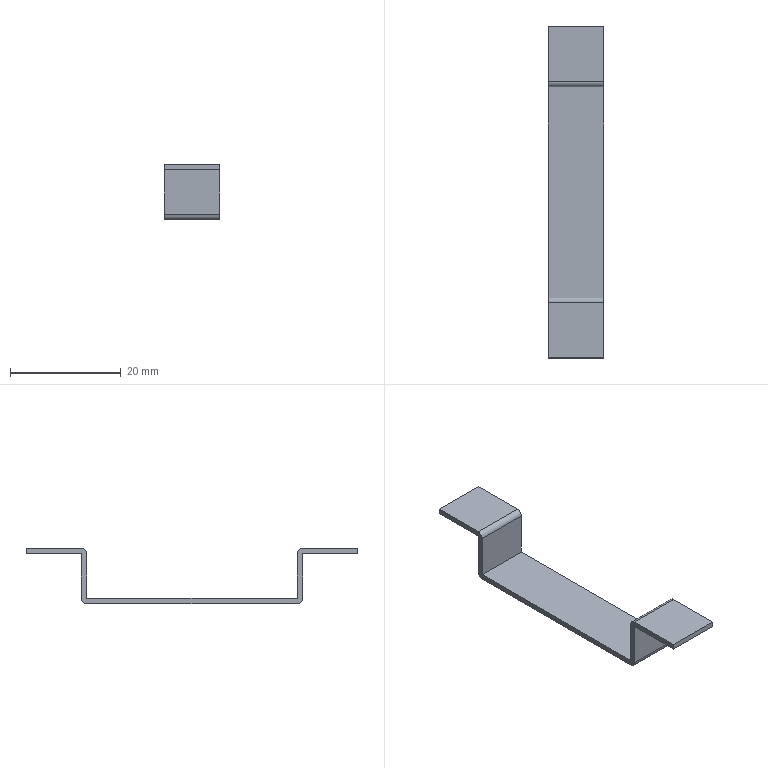Part | STEP file | 1 solid | 18 faces | box 10 x 60 x 10 mm | volume 771.555 mm3 | plane 14 | cylinder 4 | commonest cylinder face diameters 2.004 x4
STEP:
#1=CARTESIAN_POINT('',(0.,0.,0.));
#2=DIRECTION('',(0.,0.,1.));
#3=DIRECTION('',(1.,0.,0.));
#4=AXIS2_PLACEMENT_3D('',#1,#2,#3);
#5=CARTESIAN_POINT('',(-1090.573,5240.831,264.646));
#6=VERTEX_POINT('',#5);
#7=CARTESIAN_POINT('',(-1090.573,5240.832,272.643));
#8=VERTEX_POINT('',#7);
#9=CARTESIAN_POINT('',(-1090.573,5240.831,264.646));
#10=DIRECTION('',(0.,0.00008336,1.));
#11=VECTOR('',#10,1.);
#12=LINE('',#9,#11);
#13=CARTESIAN_POINT('',(-1090.573,5240.831,263.644));
#14=DIRECTION('',(1.,0.,0.));
#15=DIRECTION('',(0.,0.,1.));
#16=AXIS2_PLACEMENT_3D('',#13,#14,#15);
#17=PLANE('',#16);
#18=CARTESIAN_POINT('',(1.002,0.));
#19=DIRECTION('',(1.,-0.00008336));
#20=VECTOR('',#19,1.);
#21=LINE('',#18,#20);
#22=(GEOMETRIC_REPRESENTATION_CONTEXT(2)PARAMETRIC_REPRESENTATION_CONTEXT()REPRESENTATION_CONTEXT('',''));
#23=DEFINITIONAL_REPRESENTATION('',(#21),#22);
#24=PCURVE('',#17,#23);
#25=CARTESIAN_POINT('',(0.,5240.831,398.059));
#26=DIRECTION('',(0.,-1.,0.));
#27=DIRECTION('',(0.,0.,1.));
#28=AXIS2_PLACEMENT_3D('',#25,#26,#27);
#29=PLANE('',#28);
#30=CARTESIAN_POINT('',(-133.413,1090.573));
#31=DIRECTION('',(1.,0.));
#32=VECTOR('',#31,1.);
#33=LINE('',#30,#32);
#34=(GEOMETRIC_REPRESENTATION_CONTEXT(2)PARAMETRIC_REPRESENTATION_CONTEXT()REPRESENTATION_CONTEXT('',''));
#35=DEFINITIONAL_REPRESENTATION('',(#33),#34);
#36=PCURVE('',#29,#35);
#37=SURFACE_CURVE('',#12,(#24,#36),.PCURVE_S1.);
#38=EDGE_CURVE('',#6,#8,#37,.T.);
#39=ORIENTED_EDGE('',*,*,#38,.T.);
#40=CARTESIAN_POINT('',(-1090.573,5250.831,272.644));
#41=VERTEX_POINT('',#40);
#42=CARTESIAN_POINT('',(-1090.573,5240.832,272.643));
#43=DIRECTION('',(0.,1.,0.00006667));
#44=VECTOR('',#43,1.);
#45=LINE('',#42,#44);
#46=CARTESIAN_POINT('',(8.999,-0.0006667));
#47=DIRECTION('',(0.00006667,-1.));
#48=VECTOR('',#47,1.);
#49=LINE('',#46,#48);
#50=(GEOMETRIC_REPRESENTATION_CONTEXT(2)PARAMETRIC_REPRESENTATION_CONTEXT()REPRESENTATION_CONTEXT('',''));
#51=DEFINITIONAL_REPRESENTATION('',(#49),#50);
#52=PCURVE('',#17,#51);
#53=CARTESIAN_POINT('',(0.,0.,272.644));
#54=DIRECTION('',(0.,0.,1.));
#55=DIRECTION('',(-1.,0.,0.));
#56=AXIS2_PLACEMENT_3D('',#53,#54,#55);
#57=PLANE('',#56);
#58=CARTESIAN_POINT('',(1090.573,-5240.832));
#59=DIRECTION('',(0.,-1.));
#60=VECTOR('',#59,1.);
#61=LINE('',#58,#60);
#62=(GEOMETRIC_REPRESENTATION_CONTEXT(2)PARAMETRIC_REPRESENTATION_CONTEXT()REPRESENTATION_CONTEXT('',''));
#63=DEFINITIONAL_REPRESENTATION('',(#61),#62);
#64=PCURVE('',#57,#63);
#65=SURFACE_CURVE('',#45,(#52,#64),.PCURVE_S1.);
#66=EDGE_CURVE('',#8,#41,#65,.T.);
#67=ORIENTED_EDGE('',*,*,#66,.T.);
#68=CARTESIAN_POINT('',(-1090.573,5250.831,273.644));
#69=VERTEX_POINT('',#68);
#70=CARTESIAN_POINT('',(-1090.573,5250.831,273.644));
#71=DIRECTION('',(0.,0.,-1.));
#72=VECTOR('',#71,1.);
#73=LINE('',#70,#72);
#74=CARTESIAN_POINT('',(10.,-10.));
#75=DIRECTION('',(-1.,0.));
#76=VECTOR('',#75,1.);
#77=LINE('',#74,#76);
#78=(GEOMETRIC_REPRESENTATION_CONTEXT(2)PARAMETRIC_REPRESENTATION_CONTEXT()REPRESENTATION_CONTEXT('',''));
#79=DEFINITIONAL_REPRESENTATION('',(#77),#78);
#80=PCURVE('',#17,#79);
#81=CARTESIAN_POINT('',(-1090.573,5250.831,273.644));
#82=DIRECTION('',(0.,-1.,0.));
#83=DIRECTION('',(0.,0.,1.));
#84=AXIS2_PLACEMENT_3D('',#81,#82,#83);
#85=PLANE('',#84);
#86=CARTESIAN_POINT('',(0.,0.));
#87=DIRECTION('',(-1.,0.));
#88=VECTOR('',#87,1.);
#89=LINE('',#86,#88);
#90=(GEOMETRIC_REPRESENTATION_CONTEXT(2)PARAMETRIC_REPRESENTATION_CONTEXT()REPRESENTATION_CONTEXT('',''));
#91=DEFINITIONAL_REPRESENTATION('',(#89),#90);
#92=PCURVE('',#85,#91);
#93=SURFACE_CURVE('',#73,(#80,#92),.PCURVE_S1.);
#94=EDGE_CURVE('',#69,#41,#93,.T.);
#95=ORIENTED_EDGE('',*,*,#94,.F.);
#96=CARTESIAN_POINT('',(-1090.573,5240.833,273.644));
#97=VERTEX_POINT('',#96);
#98=CARTESIAN_POINT('',(-1090.573,5240.833,273.644));
#99=DIRECTION('',(0.,1.,0.));
#100=VECTOR('',#99,1.);
#101=LINE('',#98,#100);
#102=CARTESIAN_POINT('',(10.,-0.002));
#103=DIRECTION('',(0.,-1.));
#104=VECTOR('',#103,1.);
#105=LINE('',#102,#104);
#106=(GEOMETRIC_REPRESENTATION_CONTEXT(2)PARAMETRIC_REPRESENTATION_CONTEXT()REPRESENTATION_CONTEXT('',''));
#107=DEFINITIONAL_REPRESENTATION('',(#105),#106);
#108=PCURVE('',#17,#107);
#109=CARTESIAN_POINT('',(0.,0.,273.644));
#110=DIRECTION('',(0.,0.,1.));
#111=DIRECTION('',(-1.,0.,0.));
#112=AXIS2_PLACEMENT_3D('',#109,#110,#111);
#113=PLANE('',#112);
#114=CARTESIAN_POINT('',(1090.573,-5240.833));
#115=DIRECTION('',(0.,-1.));
#116=VECTOR('',#115,1.);
#117=LINE('',#114,#116);
#118=(GEOMETRIC_REPRESENTATION_CONTEXT(2)PARAMETRIC_REPRESENTATION_CONTEXT()REPRESENTATION_CONTEXT('',''));
#119=DEFINITIONAL_REPRESENTATION('',(#117),#118);
#120=PCURVE('',#113,#119);
#121=SURFACE_CURVE('',#101,(#108,#120),.PCURVE_S1.);
#122=EDGE_CURVE('',#97,#69,#121,.T.);
#123=ORIENTED_EDGE('',*,*,#122,.F.);
#124=CARTESIAN_POINT('',(-1090.573,5239.831,272.642));
#125=VERTEX_POINT('',#124);
#126=CARTESIAN_POINT('',(-1090.573,5240.833,272.642));
#127=DIRECTION('',(-1.,0.,0.));
#128=DIRECTION('',(0.,-1.,0.));
#129=AXIS2_PLACEMENT_3D('',#126,#127,#128);
#130=CIRCLE('',#129,1.002);
#131=CARTESIAN_POINT('',(8.998,1.));
#132=CARTESIAN_POINT('',(10.734,1.));
#133=CARTESIAN_POINT('',(9.866,-0.503));
#134=CARTESIAN_POINT('',(8.998,-2.006));
#135=CARTESIAN_POINT('',(8.13,-0.503));
#136=CARTESIAN_POINT('',(7.262,1.));
#137=CARTESIAN_POINT('',(8.998,1.));
#138=(BOUNDED_CURVE()B_SPLINE_CURVE(2,(#131,#132,#133,#134,#135,#136,#137),.UNSPECIFIED.,.T.,.F.)B_SPLINE_CURVE_WITH_KNOTS((1,2,2,2,2,1),(-2.094,0.,2.094,4.189,6.283,8.378),.UNSPECIFIED.)CURVE()GEOMETRIC_REPRESENTATION_ITEM()RATIONAL_B_SPLINE_CURVE((1.,0.5,1.,0.5,1.,0.5,1.))REPRESENTATION_ITEM(''));
#139=(GEOMETRIC_REPRESENTATION_CONTEXT(2)PARAMETRIC_REPRESENTATION_CONTEXT()REPRESENTATION_CONTEXT('',''));
#140=DEFINITIONAL_REPRESENTATION('',(#138),#139);
#141=PCURVE('',#17,#140);
#142=CARTESIAN_POINT('',(-1090.573,5240.833,272.642));
#143=DIRECTION('',(1.,0.,0.));
#144=DIRECTION('',(0.,1.,0.));
#145=AXIS2_PLACEMENT_3D('',#142,#143,#144);
#146=CYLINDRICAL_SURFACE('',#145,1.002);
#147=CARTESIAN_POINT('',(3.142,0.));
#148=DIRECTION('',(-1.,0.));
#149=VECTOR('',#148,1.);
#150=LINE('',#147,#149);
#151=(GEOMETRIC_REPRESENTATION_CONTEXT(2)PARAMETRIC_REPRESENTATION_CONTEXT()REPRESENTATION_CONTEXT('',''));
#152=DEFINITIONAL_REPRESENTATION('',(#150),#151);
#153=PCURVE('',#146,#152);
#154=SURFACE_CURVE('',#130,(#141,#153),.PCURVE_S1.);
#155=EDGE_CURVE('',#125,#97,#154,.T.);
#156=ORIENTED_EDGE('',*,*,#155,.F.);
#157=CARTESIAN_POINT('',(-1090.573,5239.831,264.644));
#158=VERTEX_POINT('',#157);
#159=CARTESIAN_POINT('',(-1090.573,5239.831,264.644));
#160=DIRECTION('',(0.,0.00008336,1.));
#161=VECTOR('',#160,1.);
#162=LINE('',#159,#161);
#163=CARTESIAN_POINT('',(1.001,1.001));
#164=DIRECTION('',(1.,-0.00008336));
#165=VECTOR('',#164,1.);
#166=LINE('',#163,#165);
#167=(GEOMETRIC_REPRESENTATION_CONTEXT(2)PARAMETRIC_REPRESENTATION_CONTEXT()REPRESENTATION_CONTEXT('',''));
#168=DEFINITIONAL_REPRESENTATION('',(#166),#167);
#169=PCURVE('',#17,#168);
#170=CARTESIAN_POINT('',(0.,5239.831,398.059));
#171=DIRECTION('',(0.,-1.,0.));
#172=DIRECTION('',(0.,0.,1.));
#173=AXIS2_PLACEMENT_3D('',#170,#171,#172);
#174=PLANE('',#173);
#175=CARTESIAN_POINT('',(-133.414,1090.573));
#176=DIRECTION('',(1.,0.));
#177=VECTOR('',#176,1.);
#178=LINE('',#175,#177);
#179=(GEOMETRIC_REPRESENTATION_CONTEXT(2)PARAMETRIC_REPRESENTATION_CONTEXT()REPRESENTATION_CONTEXT('',''));
#180=DEFINITIONAL_REPRESENTATION('',(#178),#179);
#181=PCURVE('',#174,#180);
#182=SURFACE_CURVE('',#162,(#169,#181),.PCURVE_S1.);
#183=EDGE_CURVE('',#158,#125,#182,.T.);
#184=ORIENTED_EDGE('',*,*,#183,.F.);
#185=CARTESIAN_POINT('',(-1090.573,5201.832,264.644));
#186=VERTEX_POINT('',#185);
#187=CARTESIAN_POINT('',(-1090.573,5239.831,264.644));
#188=DIRECTION('',(0.,-1.,0.));
#189=VECTOR('',#188,1.);
#190=LINE('',#187,#189);
#191=CARTESIAN_POINT('',(1.001,1.001));
#192=DIRECTION('',(0.,1.));
#193=VECTOR('',#192,1.);
#194=LINE('',#191,#193);
#195=(GEOMETRIC_REPRESENTATION_CONTEXT(2)PARAMETRIC_REPRESENTATION_CONTEXT()REPRESENTATION_CONTEXT('',''));
#196=DEFINITIONAL_REPRESENTATION('',(#194),#195);
#197=PCURVE('',#17,#196);
#198=CARTESIAN_POINT('',(0.,0.,264.644));
#199=DIRECTION('',(0.,0.,-1.));
#200=DIRECTION('',(1.,0.,0.));
#201=AXIS2_PLACEMENT_3D('',#198,#199,#200);
#202=PLANE('',#201);
#203=CARTESIAN_POINT('',(-1090.573,-5239.831));
#204=DIRECTION('',(0.,1.));
#205=VECTOR('',#204,1.);
#206=LINE('',#203,#205);
#207=(GEOMETRIC_REPRESENTATION_CONTEXT(2)PARAMETRIC_REPRESENTATION_CONTEXT()REPRESENTATION_CONTEXT('',''));
#208=DEFINITIONAL_REPRESENTATION('',(#206),#207);
#209=PCURVE('',#202,#208);
#210=SURFACE_CURVE('',#190,(#197,#209),.PCURVE_S1.);
#211=EDGE_CURVE('',#158,#186,#210,.T.);
#212=ORIENTED_EDGE('',*,*,#211,.T.);
#213=CARTESIAN_POINT('',(-1090.573,5201.831,272.642));
#214=VERTEX_POINT('',#213);
#215=CARTESIAN_POINT('',(-1090.573,5201.832,264.644));
#216=DIRECTION('',(0.,-0.00008336,1.));
#217=VECTOR('',#216,1.);
#218=LINE('',#215,#217);
#219=CARTESIAN_POINT('',(1.001,38.999));
#220=DIRECTION('',(1.,0.00008336));
#221=VECTOR('',#220,1.);
#222=LINE('',#219,#221);
#223=(GEOMETRIC_REPRESENTATION_CONTEXT(2)PARAMETRIC_REPRESENTATION_CONTEXT()REPRESENTATION_CONTEXT('',''));
#224=DEFINITIONAL_REPRESENTATION('',(#222),#223);
#225=PCURVE('',#17,#224);
#226=CARTESIAN_POINT('',(0.,5201.831,398.059));
#227=DIRECTION('',(0.,-1.,0.));
#228=DIRECTION('',(0.,0.,1.));
#229=AXIS2_PLACEMENT_3D('',#226,#227,#228);
#230=PLANE('',#229);
#231=CARTESIAN_POINT('',(-133.414,1090.573));
#232=DIRECTION('',(1.,0.));
#233=VECTOR('',#232,1.);
#234=LINE('',#231,#233);
#235=(GEOMETRIC_REPRESENTATION_CONTEXT(2)PARAMETRIC_REPRESENTATION_CONTEXT()REPRESENTATION_CONTEXT('',''));
#236=DEFINITIONAL_REPRESENTATION('',(#234),#235);
#237=PCURVE('',#230,#236);
#238=SURFACE_CURVE('',#218,(#225,#237),.PCURVE_S1.);
#239=EDGE_CURVE('',#186,#214,#238,.T.);
#240=ORIENTED_EDGE('',*,*,#239,.T.);
#241=CARTESIAN_POINT('',(-1090.573,5200.829,273.644));
#242=VERTEX_POINT('',#241);
#243=CARTESIAN_POINT('',(-1090.573,5200.829,272.642));
#244=DIRECTION('',(-1.,0.,0.));
#245=DIRECTION('',(0.,0.,1.));
#246=AXIS2_PLACEMENT_3D('',#243,#244,#245);
#247=CIRCLE('',#246,1.002);
#248=CARTESIAN_POINT('',(10.,40.002));
#249=CARTESIAN_POINT('',(10.,38.266));
#250=CARTESIAN_POINT('',(8.497,39.134));
#251=CARTESIAN_POINT('',(6.994,40.002));
#252=CARTESIAN_POINT('',(8.497,40.87));
#253=CARTESIAN_POINT('',(10.,41.738));
#254=CARTESIAN_POINT('',(10.,40.002));
#255=(BOUNDED_CURVE()B_SPLINE_CURVE(2,(#248,#249,#250,#251,#252,#253,#254),.UNSPECIFIED.,.T.,.F.)B_SPLINE_CURVE_WITH_KNOTS((1,2,2,2,2,1),(-2.094,0.,2.094,4.189,6.283,8.378),.UNSPECIFIED.)CURVE()GEOMETRIC_REPRESENTATION_ITEM()RATIONAL_B_SPLINE_CURVE((1.,0.5,1.,0.5,1.,0.5,1.))REPRESENTATION_ITEM(''));
#256=(GEOMETRIC_REPRESENTATION_CONTEXT(2)PARAMETRIC_REPRESENTATION_CONTEXT()REPRESENTATION_CONTEXT('',''));
#257=DEFINITIONAL_REPRESENTATION('',(#255),#256);
#258=PCURVE('',#17,#257);
#259=CARTESIAN_POINT('',(-1080.573,5200.829,272.642));
#260=DIRECTION('',(-1.,0.,0.));
#261=DIRECTION('',(0.,-1.,0.));
#262=AXIS2_PLACEMENT_3D('',#259,#260,#261);
#263=CYLINDRICAL_SURFACE('',#262,1.002);
#264=CARTESIAN_POINT('',(1.571,10.));
#265=DIRECTION('',(1.,0.));
#266=VECTOR('',#265,1.);
#267=LINE('',#264,#266);
#268=(GEOMETRIC_REPRESENTATION_CONTEXT(2)PARAMETRIC_REPRESENTATION_CONTEXT()REPRESENTATION_CONTEXT('',''));
#269=DEFINITIONAL_REPRESENTATION('',(#267),#268);
#270=PCURVE('',#263,#269);
#271=SURFACE_CURVE('',#247,(#258,#270),.PCURVE_S1.);
#272=EDGE_CURVE('',#242,#214,#271,.T.);
#273=ORIENTED_EDGE('',*,*,#272,.F.);
#274=CARTESIAN_POINT('',(-1090.573,5190.831,273.644));
#275=VERTEX_POINT('',#274);
#276=CARTESIAN_POINT('',(-1090.573,5200.829,273.644));
#277=DIRECTION('',(0.,-1.,0.));
#278=VECTOR('',#277,1.);
#279=LINE('',#276,#278);
#280=CARTESIAN_POINT('',(10.,40.002));
#281=DIRECTION('',(0.,1.));
#282=VECTOR('',#281,1.);
#283=LINE('',#280,#282);
#284=(GEOMETRIC_REPRESENTATION_CONTEXT(2)PARAMETRIC_REPRESENTATION_CONTEXT()REPRESENTATION_CONTEXT('',''));
#285=DEFINITIONAL_REPRESENTATION('',(#283),#284);
#286=PCURVE('',#17,#285);
#287=CARTESIAN_POINT('',(0.,0.,273.644));
#288=DIRECTION('',(0.,0.,-1.));
#289=DIRECTION('',(1.,0.,0.));
#290=AXIS2_PLACEMENT_3D('',#287,#288,#289);
#291=PLANE('',#290);
#292=CARTESIAN_POINT('',(-1090.573,-5200.829));
#293=DIRECTION('',(0.,1.));
#294=VECTOR('',#293,1.);
#295=LINE('',#292,#294);
#296=(GEOMETRIC_REPRESENTATION_CONTEXT(2)PARAMETRIC_REPRESENTATION_CONTEXT()REPRESENTATION_CONTEXT('',''));
#297=DEFINITIONAL_REPRESENTATION('',(#295),#296);
#298=PCURVE('',#291,#297);
#299=SURFACE_CURVE('',#279,(#286,#298),.PCURVE_S1.);
#300=EDGE_CURVE('',#242,#275,#299,.T.);
#301=ORIENTED_EDGE('',*,*,#300,.T.);
#302=CARTESIAN_POINT('',(-1090.573,5190.831,272.644));
#303=VERTEX_POINT('',#302);
#304=CARTESIAN_POINT('',(-1090.573,5190.831,273.644));
#305=DIRECTION('',(0.,0.,-1.));
#306=VECTOR('',#305,1.);
#307=LINE('',#304,#306);
#308=CARTESIAN_POINT('',(10.,50.));
#309=DIRECTION('',(-1.,0.));
#310=VECTOR('',#309,1.);
#311=LINE('',#308,#310);
#312=(GEOMETRIC_REPRESENTATION_CONTEXT(2)PARAMETRIC_REPRESENTATION_CONTEXT()REPRESENTATION_CONTEXT('',''));
#313=DEFINITIONAL_REPRESENTATION('',(#311),#312);
#314=PCURVE('',#17,#313);
#315=CARTESIAN_POINT('',(-1090.573,5190.831,273.644));
#316=DIRECTION('',(0.,-1.,0.));
#317=DIRECTION('',(0.,0.,1.));
#318=AXIS2_PLACEMENT_3D('',#315,#316,#317);
#319=PLANE('',#318);
#320=CARTESIAN_POINT('',(0.,0.));
#321=DIRECTION('',(-1.,0.));
#322=VECTOR('',#321,1.);
#323=LINE('',#320,#322);
#324=(GEOMETRIC_REPRESENTATION_CONTEXT(2)PARAMETRIC_REPRESENTATION_CONTEXT()REPRESENTATION_CONTEXT('',''));
#325=DEFINITIONAL_REPRESENTATION('',(#323),#324);
#326=PCURVE('',#319,#325);
#327=SURFACE_CURVE('',#307,(#314,#326),.PCURVE_S1.);
#328=EDGE_CURVE('',#275,#303,#327,.T.);
#329=ORIENTED_EDGE('',*,*,#328,.T.);
#330=CARTESIAN_POINT('',(-1090.573,5200.831,272.643));
#331=VERTEX_POINT('',#330);
#332=CARTESIAN_POINT('',(-1090.573,5200.831,272.643));
#333=DIRECTION('',(0.,-1.,0.00006667));
#334=VECTOR('',#333,1.);
#335=LINE('',#332,#334);
#336=CARTESIAN_POINT('',(8.999,40.001));
#337=DIRECTION('',(0.00006667,1.));
#338=VECTOR('',#337,1.);
#339=LINE('',#336,#338);
#340=(GEOMETRIC_REPRESENTATION_CONTEXT(2)PARAMETRIC_REPRESENTATION_CONTEXT()REPRESENTATION_CONTEXT('',''));
#341=DEFINITIONAL_REPRESENTATION('',(#339),#340);
#342=PCURVE('',#17,#341);
#343=CARTESIAN_POINT('',(0.,0.,272.644));
#344=DIRECTION('',(0.,0.,-1.));
#345=DIRECTION('',(1.,0.,0.));
#346=AXIS2_PLACEMENT_3D('',#343,#344,#345);
#347=PLANE('',#346);
#348=CARTESIAN_POINT('',(-1090.573,-5200.831));
#349=DIRECTION('',(0.,1.));
#350=VECTOR('',#349,1.);
#351=LINE('',#348,#350);
#352=(GEOMETRIC_REPRESENTATION_CONTEXT(2)PARAMETRIC_REPRESENTATION_CONTEXT()REPRESENTATION_CONTEXT('',''));
#353=DEFINITIONAL_REPRESENTATION('',(#351),#352);
#354=PCURVE('',#347,#353);
#355=SURFACE_CURVE('',#335,(#342,#354),.PCURVE_S1.);
#356=EDGE_CURVE('',#331,#303,#355,.T.);
#357=ORIENTED_EDGE('',*,*,#356,.F.);
#358=CARTESIAN_POINT('',(-1090.573,5200.831,264.646));
#359=VERTEX_POINT('',#358);
#360=CARTESIAN_POINT('',(-1090.573,5200.831,264.646));
#361=DIRECTION('',(0.,-0.00008336,1.));
#362=VECTOR('',#361,1.);
#363=LINE('',#360,#362);
#364=CARTESIAN_POINT('',(1.002,40.));
#365=DIRECTION('',(1.,0.00008336));
#366=VECTOR('',#365,1.);
#367=LINE('',#364,#366);
#368=(GEOMETRIC_REPRESENTATION_CONTEXT(2)PARAMETRIC_REPRESENTATION_CONTEXT()REPRESENTATION_CONTEXT('',''));
#369=DEFINITIONAL_REPRESENTATION('',(#367),#368);
#370=PCURVE('',#17,#369);
#371=CARTESIAN_POINT('',(0.,5200.831,398.059));
#372=DIRECTION('',(0.,-1.,0.));
#373=DIRECTION('',(0.,0.,1.));
#374=AXIS2_PLACEMENT_3D('',#371,#372,#373);
#375=PLANE('',#374);
#376=CARTESIAN_POINT('',(-133.413,1090.573));
#377=DIRECTION('',(1.,0.));
#378=VECTOR('',#377,1.);
#379=LINE('',#376,#378);
#380=(GEOMETRIC_REPRESENTATION_CONTEXT(2)PARAMETRIC_REPRESENTATION_CONTEXT()REPRESENTATION_CONTEXT('',''));
#381=DEFINITIONAL_REPRESENTATION('',(#379),#380);
#382=PCURVE('',#375,#381);
#383=SURFACE_CURVE('',#363,(#370,#382),.PCURVE_S1.);
#384=EDGE_CURVE('',#359,#331,#383,.T.);
#385=ORIENTED_EDGE('',*,*,#384,.F.);
#386=CARTESIAN_POINT('',(-1090.573,5201.833,263.644));
#387=VERTEX_POINT('',#386);
#388=CARTESIAN_POINT('',(-1090.573,5201.833,264.646));
#389=DIRECTION('',(-1.,0.,0.));
#390=DIRECTION('',(0.,0.,-1.));
#391=AXIS2_PLACEMENT_3D('',#388,#389,#390);
#392=CIRCLE('',#391,1.002);
#393=CARTESIAN_POINT('',(0.,38.998));
#394=CARTESIAN_POINT('',(0.,40.734));
#395=CARTESIAN_POINT('',(1.503,39.866));
#396=CARTESIAN_POINT('',(3.006,38.998));
#397=CARTESIAN_POINT('',(1.503,38.13));
#398=CARTESIAN_POINT('',(0.,37.262));
#399=CARTESIAN_POINT('',(0.,38.998));
#400=(BOUNDED_CURVE()B_SPLINE_CURVE(2,(#393,#394,#395,#396,#397,#398,#399),.UNSPECIFIED.,.T.,.F.)B_SPLINE_CURVE_WITH_KNOTS((1,2,2,2,2,1),(-2.094,0.,2.094,4.189,6.283,8.378),.UNSPECIFIED.)CURVE()GEOMETRIC_REPRESENTATION_ITEM()RATIONAL_B_SPLINE_CURVE((1.,0.5,1.,0.5,1.,0.5,1.))REPRESENTATION_ITEM(''));
#401=(GEOMETRIC_REPRESENTATION_CONTEXT(2)PARAMETRIC_REPRESENTATION_CONTEXT()REPRESENTATION_CONTEXT('',''));
#402=DEFINITIONAL_REPRESENTATION('',(#400),#401);
#403=PCURVE('',#17,#402);
#404=CARTESIAN_POINT('',(-1090.573,5201.833,264.646));
#405=DIRECTION('',(1.,0.,0.));
#406=DIRECTION('',(0.,0.,1.));
#407=AXIS2_PLACEMENT_3D('',#404,#405,#406);
#408=CYLINDRICAL_SURFACE('',#407,1.002);
#409=CARTESIAN_POINT('',(3.142,0.));
#410=DIRECTION('',(-1.,0.));
#411=VECTOR('',#410,1.);
#412=LINE('',#409,#411);
#413=(GEOMETRIC_REPRESENTATION_CONTEXT(2)PARAMETRIC_REPRESENTATION_CONTEXT()REPRESENTATION_CONTEXT('',''));
#414=DEFINITIONAL_REPRESENTATION('',(#412),#413);
#415=PCURVE('',#408,#414);
#416=SURFACE_CURVE('',#392,(#403,#415),.PCURVE_S1.);
#417=EDGE_CURVE('',#387,#359,#416,.T.);
#418=ORIENTED_EDGE('',*,*,#417,.F.);
#419=CARTESIAN_POINT('',(-1090.573,5239.829,263.644));
#420=VERTEX_POINT('',#419);
#421=CARTESIAN_POINT('',(-1090.573,5239.829,263.644));
#422=DIRECTION('',(0.,-1.,0.));
#423=VECTOR('',#422,1.);
#424=LINE('',#421,#423);
#425=CARTESIAN_POINT('',(0.,1.002));
#426=DIRECTION('',(0.,1.));
#427=VECTOR('',#426,1.);
#428=LINE('',#425,#427);
#429=(GEOMETRIC_REPRESENTATION_CONTEXT(2)PARAMETRIC_REPRESENTATION_CONTEXT()REPRESENTATION_CONTEXT('',''));
#430=DEFINITIONAL_REPRESENTATION('',(#428),#429);
#431=PCURVE('',#17,#430);
#432=CARTESIAN_POINT('',(0.,0.,263.644));
#433=DIRECTION('',(0.,0.,-1.));
#434=DIRECTION('',(1.,0.,0.));
#435=AXIS2_PLACEMENT_3D('',#432,#433,#434);
#436=PLANE('',#435);
#437=CARTESIAN_POINT('',(-1090.573,-5239.829));
#438=DIRECTION('',(0.,1.));
#439=VECTOR('',#438,1.);
#440=LINE('',#437,#439);
#441=(GEOMETRIC_REPRESENTATION_CONTEXT(2)PARAMETRIC_REPRESENTATION_CONTEXT()REPRESENTATION_CONTEXT('',''));
#442=DEFINITIONAL_REPRESENTATION('',(#440),#441);
#443=PCURVE('',#436,#442);
#444=SURFACE_CURVE('',#424,(#431,#443),.PCURVE_S1.);
#445=EDGE_CURVE('',#420,#387,#444,.T.);
#446=ORIENTED_EDGE('',*,*,#445,.F.);
#447=CARTESIAN_POINT('',(-1090.573,5239.829,264.646));
#448=DIRECTION('',(-1.,0.,0.));
#449=DIRECTION('',(0.,1.,0.));
#450=AXIS2_PLACEMENT_3D('',#447,#448,#449);
#451=CIRCLE('',#450,1.002);
#452=CARTESIAN_POINT('',(1.002,0.));
#453=CARTESIAN_POINT('',(-0.7335,0.));
#454=CARTESIAN_POINT('',(0.1342,1.503));
#455=CARTESIAN_POINT('',(1.002,3.006));
#456=CARTESIAN_POINT('',(1.87,1.503));
#457=CARTESIAN_POINT('',(2.738,0.));
#458=CARTESIAN_POINT('',(1.002,0.));
#459=(BOUNDED_CURVE()B_SPLINE_CURVE(2,(#452,#453,#454,#455,#456,#457,#458),.UNSPECIFIED.,.T.,.F.)B_SPLINE_CURVE_WITH_KNOTS((1,2,2,2,2,1),(-2.094,0.,2.094,4.189,6.283,8.378),.UNSPECIFIED.)CURVE()GEOMETRIC_REPRESENTATION_ITEM()RATIONAL_B_SPLINE_CURVE((1.,0.5,1.,0.5,1.,0.5,1.))REPRESENTATION_ITEM(''));
#460=(GEOMETRIC_REPRESENTATION_CONTEXT(2)PARAMETRIC_REPRESENTATION_CONTEXT()REPRESENTATION_CONTEXT('',''));
#461=DEFINITIONAL_REPRESENTATION('',(#459),#460);
#462=PCURVE('',#17,#461);
#463=CARTESIAN_POINT('',(-1080.573,5239.829,264.646));
#464=DIRECTION('',(-1.,0.,0.));
#465=DIRECTION('',(0.,0.,1.));
#466=AXIS2_PLACEMENT_3D('',#463,#464,#465);
#467=CYLINDRICAL_SURFACE('',#466,1.002);
#468=CARTESIAN_POINT('',(1.571,10.));
#469=DIRECTION('',(1.,0.));
#470=VECTOR('',#469,1.);
#471=LINE('',#468,#470);
#472=(GEOMETRIC_REPRESENTATION_CONTEXT(2)PARAMETRIC_REPRESENTATION_CONTEXT()REPRESENTATION_CONTEXT('',''));
#473=DEFINITIONAL_REPRESENTATION('',(#471),#472);
#474=PCURVE('',#467,#473);
#475=SURFACE_CURVE('',#451,(#462,#474),.PCURVE_S1.);
#476=EDGE_CURVE('',#6,#420,#475,.T.);
#477=ORIENTED_EDGE('',*,*,#476,.F.);
#478=EDGE_LOOP('',(#39,#67,#95,#123,#156,#184,#212,#240,#273,#301,#329,#357,#385,#418,#446,#477));
#479=FACE_BOUND('',#478,.F.);
#480=ADVANCED_FACE('',(#479),#17,.F.);
#481=CARTESIAN_POINT('',(-1080.573,5240.832,272.643));
#482=VERTEX_POINT('',#481);
#483=CARTESIAN_POINT('',(-1090.573,5240.832,272.643));
#484=DIRECTION('',(1.,0.,0.));
#485=VECTOR('',#484,1.);
#486=LINE('',#483,#485);
#487=CARTESIAN_POINT('',(-125.416,1090.573));
#488=DIRECTION('',(0.,-1.));
#489=VECTOR('',#488,1.);
#490=LINE('',#487,#489);
#491=(GEOMETRIC_REPRESENTATION_CONTEXT(2)PARAMETRIC_REPRESENTATION_CONTEXT()REPRESENTATION_CONTEXT('',''));
#492=DEFINITIONAL_REPRESENTATION('',(#490),#491);
#493=PCURVE('',#29,#492);
#494=CARTESIAN_POINT('',(1090.573,-5240.832));
#495=DIRECTION('',(-1.,0.));
#496=VECTOR('',#495,1.);
#497=LINE('',#494,#496);
#498=(GEOMETRIC_REPRESENTATION_CONTEXT(2)PARAMETRIC_REPRESENTATION_CONTEXT()REPRESENTATION_CONTEXT('',''));
#499=DEFINITIONAL_REPRESENTATION('',(#497),#498);
#500=PCURVE('',#57,#499);
#501=SURFACE_CURVE('',#486,(#493,#500),.PCURVE_S1.);
#502=EDGE_CURVE('',#8,#482,#501,.T.);
#503=ORIENTED_EDGE('',*,*,#502,.F.);
#504=ORIENTED_EDGE('',*,*,#38,.F.);
#505=CARTESIAN_POINT('',(-1080.573,5240.831,264.646));
#506=VERTEX_POINT('',#505);
#507=CARTESIAN_POINT('',(-1090.573,5240.831,264.646));
#508=DIRECTION('',(1.,0.,0.));
#509=VECTOR('',#508,1.);
#510=LINE('',#507,#509);
#511=CARTESIAN_POINT('',(-133.413,1090.573));
#512=DIRECTION('',(0.,-1.));
#513=VECTOR('',#512,1.);
#514=LINE('',#511,#513);
#515=(GEOMETRIC_REPRESENTATION_CONTEXT(2)PARAMETRIC_REPRESENTATION_CONTEXT()REPRESENTATION_CONTEXT('',''));
#516=DEFINITIONAL_REPRESENTATION('',(#514),#515);
#517=PCURVE('',#29,#516);
#518=CARTESIAN_POINT('',(1.571,10.));
#519=DIRECTION('',(0.,-1.));
#520=VECTOR('',#519,1.);
#521=LINE('',#518,#520);
#522=(GEOMETRIC_REPRESENTATION_CONTEXT(2)PARAMETRIC_REPRESENTATION_CONTEXT()REPRESENTATION_CONTEXT('',''));
#523=DEFINITIONAL_REPRESENTATION('',(#521),#522);
#524=PCURVE('',#467,#523);
#525=SURFACE_CURVE('',#510,(#517,#524),.PCURVE_S1.);
#526=EDGE_CURVE('',#6,#506,#525,.T.);
#527=ORIENTED_EDGE('',*,*,#526,.T.);
#528=CARTESIAN_POINT('',(-1080.573,5240.832,272.643));
#529=DIRECTION('',(0.,-0.00008336,-1.));
#530=VECTOR('',#529,1.);
#531=LINE('',#528,#530);
#532=CARTESIAN_POINT('',(-125.416,1080.573));
#533=DIRECTION('',(-1.,0.));
#534=VECTOR('',#533,1.);
#535=LINE('',#532,#534);
#536=(GEOMETRIC_REPRESENTATION_CONTEXT(2)PARAMETRIC_REPRESENTATION_CONTEXT()REPRESENTATION_CONTEXT('',''));
#537=DEFINITIONAL_REPRESENTATION('',(#535),#536);
#538=PCURVE('',#29,#537);
#539=CARTESIAN_POINT('',(-1080.573,5200.831,263.644));
#540=DIRECTION('',(-1.,0.,0.));
#541=DIRECTION('',(0.,0.,-1.));
#542=AXIS2_PLACEMENT_3D('',#539,#540,#541);
#543=PLANE('',#542);
#544=CARTESIAN_POINT('',(-8.999,-40.001));
#545=DIRECTION('',(1.,0.00008336));
#546=VECTOR('',#545,1.);
#547=LINE('',#544,#546);
#548=(GEOMETRIC_REPRESENTATION_CONTEXT(2)PARAMETRIC_REPRESENTATION_CONTEXT()REPRESENTATION_CONTEXT('',''));
#549=DEFINITIONAL_REPRESENTATION('',(#547),#548);
#550=PCURVE('',#543,#549);
#551=SURFACE_CURVE('',#531,(#538,#550),.PCURVE_S1.);
#552=EDGE_CURVE('',#482,#506,#551,.T.);
#553=ORIENTED_EDGE('',*,*,#552,.F.);
#554=EDGE_LOOP('',(#503,#504,#527,#553));
#555=FACE_BOUND('',#554,.F.);
#556=ADVANCED_FACE('',(#555),#29,.F.);
#557=ORIENTED_EDGE('',*,*,#502,.T.);
#558=CARTESIAN_POINT('',(-1080.573,5250.831,272.644));
#559=VERTEX_POINT('',#558);
#560=CARTESIAN_POINT('',(-1080.573,5250.831,272.644));
#561=DIRECTION('',(0.,-1.,-0.00006667));
#562=VECTOR('',#561,1.);
#563=LINE('',#560,#562);
#564=CARTESIAN_POINT('',(1080.573,-5250.831));
#565=DIRECTION('',(0.,1.));
#566=VECTOR('',#565,1.);
#567=LINE('',#564,#566);
#568=(GEOMETRIC_REPRESENTATION_CONTEXT(2)PARAMETRIC_REPRESENTATION_CONTEXT()REPRESENTATION_CONTEXT('',''));
#569=DEFINITIONAL_REPRESENTATION('',(#567),#568);
#570=PCURVE('',#57,#569);
#571=CARTESIAN_POINT('',(-9.,-50.));
#572=DIRECTION('',(0.00006667,1.));
#573=VECTOR('',#572,1.);
#574=LINE('',#571,#573);
#575=(GEOMETRIC_REPRESENTATION_CONTEXT(2)PARAMETRIC_REPRESENTATION_CONTEXT()REPRESENTATION_CONTEXT('',''));
#576=DEFINITIONAL_REPRESENTATION('',(#574),#575);
#577=PCURVE('',#543,#576);
#578=SURFACE_CURVE('',#563,(#570,#577),.PCURVE_S1.);
#579=EDGE_CURVE('',#559,#482,#578,.T.);
#580=ORIENTED_EDGE('',*,*,#579,.F.);
#581=CARTESIAN_POINT('',(-1090.573,5250.831,272.644));
#582=DIRECTION('',(1.,0.,0.));
#583=VECTOR('',#582,1.);
#584=LINE('',#581,#583);
#585=CARTESIAN_POINT('',(1090.573,-5250.831));
#586=DIRECTION('',(-1.,0.));
#587=VECTOR('',#586,1.);
#588=LINE('',#585,#587);
#589=(GEOMETRIC_REPRESENTATION_CONTEXT(2)PARAMETRIC_REPRESENTATION_CONTEXT()REPRESENTATION_CONTEXT('',''));
#590=DEFINITIONAL_REPRESENTATION('',(#588),#589);
#591=PCURVE('',#57,#590);
#592=CARTESIAN_POINT('',(-1.,0.));
#593=DIRECTION('',(0.,-1.));
#594=VECTOR('',#593,1.);
#595=LINE('',#592,#594);
#596=(GEOMETRIC_REPRESENTATION_CONTEXT(2)PARAMETRIC_REPRESENTATION_CONTEXT()REPRESENTATION_CONTEXT('',''));
#597=DEFINITIONAL_REPRESENTATION('',(#595),#596);
#598=PCURVE('',#85,#597);
#599=SURFACE_CURVE('',#584,(#591,#598),.PCURVE_S1.);
#600=EDGE_CURVE('',#41,#559,#599,.T.);
#601=ORIENTED_EDGE('',*,*,#600,.F.);
#602=ORIENTED_EDGE('',*,*,#66,.F.);
#603=EDGE_LOOP('',(#557,#580,#601,#602));
#604=FACE_BOUND('',#603,.F.);
#605=ADVANCED_FACE('',(#604),#57,.F.);
#606=CARTESIAN_POINT('',(-1080.573,5239.831,272.642));
#607=VERTEX_POINT('',#606);
#608=CARTESIAN_POINT('',(-1080.573,5239.831,264.644));
#609=VERTEX_POINT('',#608);
#610=CARTESIAN_POINT('',(-1080.573,5239.831,272.642));
#611=DIRECTION('',(0.,-0.00008336,-1.));
#612=VECTOR('',#611,1.);
#613=LINE('',#610,#612);
#614=CARTESIAN_POINT('',(-8.998,-39.));
#615=DIRECTION('',(1.,0.00008336));
#616=VECTOR('',#615,1.);
#617=LINE('',#614,#616);
#618=(GEOMETRIC_REPRESENTATION_CONTEXT(2)PARAMETRIC_REPRESENTATION_CONTEXT()REPRESENTATION_CONTEXT('',''));
#619=DEFINITIONAL_REPRESENTATION('',(#617),#618);
#620=PCURVE('',#543,#619);
#621=CARTESIAN_POINT('',(-125.417,1080.573));
#622=DIRECTION('',(-1.,0.));
#623=VECTOR('',#622,1.);
#624=LINE('',#621,#623);
#625=(GEOMETRIC_REPRESENTATION_CONTEXT(2)PARAMETRIC_REPRESENTATION_CONTEXT()REPRESENTATION_CONTEXT('',''));
#626=DEFINITIONAL_REPRESENTATION('',(#624),#625);
#627=PCURVE('',#174,#626);
#628=SURFACE_CURVE('',#613,(#620,#627),.PCURVE_S1.);
#629=EDGE_CURVE('',#607,#609,#628,.T.);
#630=ORIENTED_EDGE('',*,*,#629,.F.);
#631=CARTESIAN_POINT('',(-1080.573,5240.833,273.644));
#632=VERTEX_POINT('',#631);
#633=CARTESIAN_POINT('',(-1080.573,5240.833,272.642));
#634=DIRECTION('',(1.,0.,0.));
#635=DIRECTION('',(0.,0.,1.));
#636=AXIS2_PLACEMENT_3D('',#633,#634,#635);
#637=CIRCLE('',#636,1.002);
#638=CARTESIAN_POINT('',(-10.,-40.002));
#639=CARTESIAN_POINT('',(-10.,-38.266));
#640=CARTESIAN_POINT('',(-8.497,-39.134));
#641=CARTESIAN_POINT('',(-6.994,-40.002));
#642=CARTESIAN_POINT('',(-8.497,-40.87));
#643=CARTESIAN_POINT('',(-10.,-41.738));
#644=CARTESIAN_POINT('',(-10.,-40.002));
#645=(BOUNDED_CURVE()B_SPLINE_CURVE(2,(#638,#639,#640,#641,#642,#643,#644),.UNSPECIFIED.,.T.,.F.)B_SPLINE_CURVE_WITH_KNOTS((1,2,2,2,2,1),(-2.094,0.,2.094,4.189,6.283,8.378),.UNSPECIFIED.)CURVE()GEOMETRIC_REPRESENTATION_ITEM()RATIONAL_B_SPLINE_CURVE((1.,0.5,1.,0.5,1.,0.5,1.))REPRESENTATION_ITEM(''));
#646=(GEOMETRIC_REPRESENTATION_CONTEXT(2)PARAMETRIC_REPRESENTATION_CONTEXT()REPRESENTATION_CONTEXT('',''));
#647=DEFINITIONAL_REPRESENTATION('',(#645),#646);
#648=PCURVE('',#543,#647);
#649=CARTESIAN_POINT('',(1.571,10.));
#650=DIRECTION('',(1.,0.));
#651=VECTOR('',#650,1.);
#652=LINE('',#649,#651);
#653=(GEOMETRIC_REPRESENTATION_CONTEXT(2)PARAMETRIC_REPRESENTATION_CONTEXT()REPRESENTATION_CONTEXT('',''));
#654=DEFINITIONAL_REPRESENTATION('',(#652),#653);
#655=PCURVE('',#146,#654);
#656=SURFACE_CURVE('',#637,(#648,#655),.PCURVE_S1.);
#657=EDGE_CURVE('',#632,#607,#656,.T.);
#658=ORIENTED_EDGE('',*,*,#657,.F.);
#659=CARTESIAN_POINT('',(-1080.573,5250.831,273.644));
#660=VERTEX_POINT('',#659);
#661=CARTESIAN_POINT('',(-1080.573,5250.831,273.644));
#662=DIRECTION('',(0.,-1.,0.));
#663=VECTOR('',#662,1.);
#664=LINE('',#661,#663);
#665=CARTESIAN_POINT('',(-10.,-50.));
#666=DIRECTION('',(0.,1.));
#667=VECTOR('',#666,1.);
#668=LINE('',#665,#667);
#669=(GEOMETRIC_REPRESENTATION_CONTEXT(2)PARAMETRIC_REPRESENTATION_CONTEXT()REPRESENTATION_CONTEXT('',''));
#670=DEFINITIONAL_REPRESENTATION('',(#668),#669);
#671=PCURVE('',#543,#670);
#672=CARTESIAN_POINT('',(1080.573,-5250.831));
#673=DIRECTION('',(0.,1.));
#674=VECTOR('',#673,1.);
#675=LINE('',#672,#674);
#676=(GEOMETRIC_REPRESENTATION_CONTEXT(2)PARAMETRIC_REPRESENTATION_CONTEXT()REPRESENTATION_CONTEXT('',''));
#677=DEFINITIONAL_REPRESENTATION('',(#675),#676);
#678=PCURVE('',#113,#677);
#679=SURFACE_CURVE('',#664,(#671,#678),.PCURVE_S1.);
#680=EDGE_CURVE('',#660,#632,#679,.T.);
#681=ORIENTED_EDGE('',*,*,#680,.F.);
#682=CARTESIAN_POINT('',(-1080.573,5250.831,273.644));
#683=DIRECTION('',(0.,0.,-1.));
#684=VECTOR('',#683,1.);
#685=LINE('',#682,#684);
#686=CARTESIAN_POINT('',(-10.,-50.));
#687=DIRECTION('',(1.,0.));
#688=VECTOR('',#687,1.);
#689=LINE('',#686,#688);
#690=(GEOMETRIC_REPRESENTATION_CONTEXT(2)PARAMETRIC_REPRESENTATION_CONTEXT()REPRESENTATION_CONTEXT('',''));
#691=DEFINITIONAL_REPRESENTATION('',(#689),#690);
#692=PCURVE('',#543,#691);
#693=CARTESIAN_POINT('',(0.,-10.));
#694=DIRECTION('',(-1.,0.));
#695=VECTOR('',#694,1.);
#696=LINE('',#693,#695);
#697=(GEOMETRIC_REPRESENTATION_CONTEXT(2)PARAMETRIC_REPRESENTATION_CONTEXT()REPRESENTATION_CONTEXT('',''));
#698=DEFINITIONAL_REPRESENTATION('',(#696),#697);
#699=PCURVE('',#85,#698);
#700=SURFACE_CURVE('',#685,(#692,#699),.PCURVE_S1.);
#701=EDGE_CURVE('',#660,#559,#700,.T.);
#702=ORIENTED_EDGE('',*,*,#701,.T.);
#703=ORIENTED_EDGE('',*,*,#579,.T.);
#704=ORIENTED_EDGE('',*,*,#552,.T.);
#705=CARTESIAN_POINT('',(-1080.573,5239.829,263.644));
#706=VERTEX_POINT('',#705);
#707=CARTESIAN_POINT('',(-1080.573,5239.829,264.646));
#708=DIRECTION('',(1.,0.,0.));
#709=DIRECTION('',(0.,0.,-1.));
#710=AXIS2_PLACEMENT_3D('',#707,#708,#709);
#711=CIRCLE('',#710,1.002);
#712=CARTESIAN_POINT('',(0.,-38.998));
#713=CARTESIAN_POINT('',(0.,-40.734));
#714=CARTESIAN_POINT('',(-1.503,-39.866));
#715=CARTESIAN_POINT('',(-3.006,-38.998));
#716=CARTESIAN_POINT('',(-1.503,-38.13));
#717=CARTESIAN_POINT('',(0.,-37.262));
#718=CARTESIAN_POINT('',(0.,-38.998));
#719=(BOUNDED_CURVE()B_SPLINE_CURVE(2,(#712,#713,#714,#715,#716,#717,#718),.UNSPECIFIED.,.T.,.F.)B_SPLINE_CURVE_WITH_KNOTS((1,2,2,2,2,1),(-2.094,0.,2.094,4.189,6.283,8.378),.UNSPECIFIED.)CURVE()GEOMETRIC_REPRESENTATION_ITEM()RATIONAL_B_SPLINE_CURVE((1.,0.5,1.,0.5,1.,0.5,1.))REPRESENTATION_ITEM(''));
#720=(GEOMETRIC_REPRESENTATION_CONTEXT(2)PARAMETRIC_REPRESENTATION_CONTEXT()REPRESENTATION_CONTEXT('',''));
#721=DEFINITIONAL_REPRESENTATION('',(#719),#720);
#722=PCURVE('',#543,#721);
#723=CARTESIAN_POINT('',(3.142,0.));
#724=DIRECTION('',(-1.,0.));
#725=VECTOR('',#724,1.);
#726=LINE('',#723,#725);
#727=(GEOMETRIC_REPRESENTATION_CONTEXT(2)PARAMETRIC_REPRESENTATION_CONTEXT()REPRESENTATION_CONTEXT('',''));
#728=DEFINITIONAL_REPRESENTATION('',(#726),#727);
#729=PCURVE('',#467,#728);
#730=SURFACE_CURVE('',#711,(#722,#729),.PCURVE_S1.);
#731=EDGE_CURVE('',#706,#506,#730,.T.);
#732=ORIENTED_EDGE('',*,*,#731,.F.);
#733=CARTESIAN_POINT('',(-1080.573,5201.833,263.644));
#734=VERTEX_POINT('',#733);
#735=CARTESIAN_POINT('',(-1080.573,5201.833,263.644));
#736=DIRECTION('',(0.,1.,0.));
#737=VECTOR('',#736,1.);
#738=LINE('',#735,#737);
#739=CARTESIAN_POINT('',(0.,-1.002));
#740=DIRECTION('',(0.,-1.));
#741=VECTOR('',#740,1.);
#742=LINE('',#739,#741);
#743=(GEOMETRIC_REPRESENTATION_CONTEXT(2)PARAMETRIC_REPRESENTATION_CONTEXT()REPRESENTATION_CONTEXT('',''));
#744=DEFINITIONAL_REPRESENTATION('',(#742),#743);
#745=PCURVE('',#543,#744);
#746=CARTESIAN_POINT('',(-1080.573,-5201.833));
#747=DIRECTION('',(0.,-1.));
#748=VECTOR('',#747,1.);
#749=LINE('',#746,#748);
#750=(GEOMETRIC_REPRESENTATION_CONTEXT(2)PARAMETRIC_REPRESENTATION_CONTEXT()REPRESENTATION_CONTEXT('',''));
#751=DEFINITIONAL_REPRESENTATION('',(#749),#750);
#752=PCURVE('',#436,#751);
#753=SURFACE_CURVE('',#738,(#745,#752),.PCURVE_S1.);
#754=EDGE_CURVE('',#734,#706,#753,.T.);
#755=ORIENTED_EDGE('',*,*,#754,.F.);
#756=CARTESIAN_POINT('',(-1080.573,5200.831,264.646));
#757=VERTEX_POINT('',#756);
#758=CARTESIAN_POINT('',(-1080.573,5201.833,264.646));
#759=DIRECTION('',(1.,0.,0.));
#760=DIRECTION('',(0.,-1.,0.));
#761=AXIS2_PLACEMENT_3D('',#758,#759,#760);
#762=CIRCLE('',#761,1.002);
#763=CARTESIAN_POINT('',(-1.002,0.));
#764=CARTESIAN_POINT('',(0.7335,0.));
#765=CARTESIAN_POINT('',(-0.1342,-1.503));
#766=CARTESIAN_POINT('',(-1.002,-3.006));
#767=CARTESIAN_POINT('',(-1.87,-1.503));
#768=CARTESIAN_POINT('',(-2.738,0.));
#769=CARTESIAN_POINT('',(-1.002,0.));
#770=(BOUNDED_CURVE()B_SPLINE_CURVE(2,(#763,#764,#765,#766,#767,#768,#769),.UNSPECIFIED.,.T.,.F.)B_SPLINE_CURVE_WITH_KNOTS((1,2,2,2,2,1),(-2.094,0.,2.094,4.189,6.283,8.378),.UNSPECIFIED.)CURVE()GEOMETRIC_REPRESENTATION_ITEM()RATIONAL_B_SPLINE_CURVE((1.,0.5,1.,0.5,1.,0.5,1.))REPRESENTATION_ITEM(''));
#771=(GEOMETRIC_REPRESENTATION_CONTEXT(2)PARAMETRIC_REPRESENTATION_CONTEXT()REPRESENTATION_CONTEXT('',''));
#772=DEFINITIONAL_REPRESENTATION('',(#770),#771);
#773=PCURVE('',#543,#772);
#774=CARTESIAN_POINT('',(1.571,10.));
#775=DIRECTION('',(1.,0.));
#776=VECTOR('',#775,1.);
#777=LINE('',#774,#776);
#778=(GEOMETRIC_REPRESENTATION_CONTEXT(2)PARAMETRIC_REPRESENTATION_CONTEXT()REPRESENTATION_CONTEXT('',''));
#779=DEFINITIONAL_REPRESENTATION('',(#777),#778);
#780=PCURVE('',#408,#779);
#781=SURFACE_CURVE('',#762,(#773,#780),.PCURVE_S1.);
#782=EDGE_CURVE('',#757,#734,#781,.T.);
#783=ORIENTED_EDGE('',*,*,#782,.F.);
#784=CARTESIAN_POINT('',(-1080.573,5200.831,272.643));
#785=VERTEX_POINT('',#784);
#786=CARTESIAN_POINT('',(-1080.573,5200.831,272.643));
#787=DIRECTION('',(0.,0.00008336,-1.));
#788=VECTOR('',#787,1.);
#789=LINE('',#786,#788);
#790=CARTESIAN_POINT('',(-8.999,0.0006667));
#791=DIRECTION('',(1.,-0.00008336));
#792=VECTOR('',#791,1.);
#793=LINE('',#790,#792);
#794=(GEOMETRIC_REPRESENTATION_CONTEXT(2)PARAMETRIC_REPRESENTATION_CONTEXT()REPRESENTATION_CONTEXT('',''));
#795=DEFINITIONAL_REPRESENTATION('',(#793),#794);
#796=PCURVE('',#543,#795);
#797=CARTESIAN_POINT('',(-125.416,1080.573));
#798=DIRECTION('',(-1.,0.));
#799=VECTOR('',#798,1.);
#800=LINE('',#797,#799);
#801=(GEOMETRIC_REPRESENTATION_CONTEXT(2)PARAMETRIC_REPRESENTATION_CONTEXT()REPRESENTATION_CONTEXT('',''));
#802=DEFINITIONAL_REPRESENTATION('',(#800),#801);
#803=PCURVE('',#375,#802);
#804=SURFACE_CURVE('',#789,(#796,#803),.PCURVE_S1.);
#805=EDGE_CURVE('',#785,#757,#804,.T.);
#806=ORIENTED_EDGE('',*,*,#805,.F.);
#807=CARTESIAN_POINT('',(-1080.573,5190.831,272.644));
#808=VERTEX_POINT('',#807);
#809=CARTESIAN_POINT('',(-1080.573,5190.831,272.644));
#810=DIRECTION('',(0.,1.,-0.00006667));
#811=VECTOR('',#810,1.);
#812=LINE('',#809,#811);
#813=CARTESIAN_POINT('',(-9.,10.));
#814=DIRECTION('',(0.00006667,-1.));
#815=VECTOR('',#814,1.);
#816=LINE('',#813,#815);
#817=(GEOMETRIC_REPRESENTATION_CONTEXT(2)PARAMETRIC_REPRESENTATION_CONTEXT()REPRESENTATION_CONTEXT('',''));
#818=DEFINITIONAL_REPRESENTATION('',(#816),#817);
#819=PCURVE('',#543,#818);
#820=CARTESIAN_POINT('',(-1080.573,-5190.831));
#821=DIRECTION('',(0.,-1.));
#822=VECTOR('',#821,1.);
#823=LINE('',#820,#822);
#824=(GEOMETRIC_REPRESENTATION_CONTEXT(2)PARAMETRIC_REPRESENTATION_CONTEXT()REPRESENTATION_CONTEXT('',''));
#825=DEFINITIONAL_REPRESENTATION('',(#823),#824);
#826=PCURVE('',#347,#825);
#827=SURFACE_CURVE('',#812,(#819,#826),.PCURVE_S1.);
#828=EDGE_CURVE('',#808,#785,#827,.T.);
#829=ORIENTED_EDGE('',*,*,#828,.F.);
#830=CARTESIAN_POINT('',(-1080.573,5190.831,273.644));
#831=VERTEX_POINT('',#830);
#832=CARTESIAN_POINT('',(-1080.573,5190.831,273.644));
#833=DIRECTION('',(0.,0.,-1.));
#834=VECTOR('',#833,1.);
#835=LINE('',#832,#834);
#836=CARTESIAN_POINT('',(-10.,10.));
#837=DIRECTION('',(1.,0.));
#838=VECTOR('',#837,1.);
#839=LINE('',#836,#838);
#840=(GEOMETRIC_REPRESENTATION_CONTEXT(2)PARAMETRIC_REPRESENTATION_CONTEXT()REPRESENTATION_CONTEXT('',''));
#841=DEFINITIONAL_REPRESENTATION('',(#839),#840);
#842=PCURVE('',#543,#841);
#843=CARTESIAN_POINT('',(0.,-10.));
#844=DIRECTION('',(-1.,0.));
#845=VECTOR('',#844,1.);
#846=LINE('',#843,#845);
#847=(GEOMETRIC_REPRESENTATION_CONTEXT(2)PARAMETRIC_REPRESENTATION_CONTEXT()REPRESENTATION_CONTEXT('',''));
#848=DEFINITIONAL_REPRESENTATION('',(#846),#847);
#849=PCURVE('',#319,#848);
#850=SURFACE_CURVE('',#835,(#842,#849),.PCURVE_S1.);
#851=EDGE_CURVE('',#831,#808,#850,.T.);
#852=ORIENTED_EDGE('',*,*,#851,.F.);
#853=CARTESIAN_POINT('',(-1080.573,5200.829,273.644));
#854=VERTEX_POINT('',#853);
#855=CARTESIAN_POINT('',(-1080.573,5190.831,273.644));
#856=DIRECTION('',(0.,1.,0.));
#857=VECTOR('',#856,1.);
#858=LINE('',#855,#857);
#859=CARTESIAN_POINT('',(-10.,10.));
#860=DIRECTION('',(0.,-1.));
#861=VECTOR('',#860,1.);
#862=LINE('',#859,#861);
#863=(GEOMETRIC_REPRESENTATION_CONTEXT(2)PARAMETRIC_REPRESENTATION_CONTEXT()REPRESENTATION_CONTEXT('',''));
#864=DEFINITIONAL_REPRESENTATION('',(#862),#863);
#865=PCURVE('',#543,#864);
#866=CARTESIAN_POINT('',(-1080.573,-5190.831));
#867=DIRECTION('',(0.,-1.));
#868=VECTOR('',#867,1.);
#869=LINE('',#866,#868);
#870=(GEOMETRIC_REPRESENTATION_CONTEXT(2)PARAMETRIC_REPRESENTATION_CONTEXT()REPRESENTATION_CONTEXT('',''));
#871=DEFINITIONAL_REPRESENTATION('',(#869),#870);
#872=PCURVE('',#291,#871);
#873=SURFACE_CURVE('',#858,(#865,#872),.PCURVE_S1.);
#874=EDGE_CURVE('',#831,#854,#873,.T.);
#875=ORIENTED_EDGE('',*,*,#874,.T.);
#876=CARTESIAN_POINT('',(-1080.573,5201.831,272.642));
#877=VERTEX_POINT('',#876);
#878=CARTESIAN_POINT('',(-1080.573,5200.829,272.642));
#879=DIRECTION('',(1.,0.,0.));
#880=DIRECTION('',(0.,1.,0.));
#881=AXIS2_PLACEMENT_3D('',#878,#879,#880);
#882=CIRCLE('',#881,1.002);
#883=CARTESIAN_POINT('',(-8.998,-1.));
#884=CARTESIAN_POINT('',(-10.734,-1.));
#885=CARTESIAN_POINT('',(-9.866,0.503));
#886=CARTESIAN_POINT('',(-8.998,2.006));
#887=CARTESIAN_POINT('',(-8.13,0.503));
#888=CARTESIAN_POINT('',(-7.262,-1.));
#889=CARTESIAN_POINT('',(-8.998,-1.));
#890=(BOUNDED_CURVE()B_SPLINE_CURVE(2,(#883,#884,#885,#886,#887,#888,#889),.UNSPECIFIED.,.T.,.F.)B_SPLINE_CURVE_WITH_KNOTS((1,2,2,2,2,1),(-2.094,0.,2.094,4.189,6.283,8.378),.UNSPECIFIED.)CURVE()GEOMETRIC_REPRESENTATION_ITEM()RATIONAL_B_SPLINE_CURVE((1.,0.5,1.,0.5,1.,0.5,1.))REPRESENTATION_ITEM(''));
#891=(GEOMETRIC_REPRESENTATION_CONTEXT(2)PARAMETRIC_REPRESENTATION_CONTEXT()REPRESENTATION_CONTEXT('',''));
#892=DEFINITIONAL_REPRESENTATION('',(#890),#891);
#893=PCURVE('',#543,#892);
#894=CARTESIAN_POINT('',(3.142,0.));
#895=DIRECTION('',(-1.,0.));
#896=VECTOR('',#895,1.);
#897=LINE('',#894,#896);
#898=(GEOMETRIC_REPRESENTATION_CONTEXT(2)PARAMETRIC_REPRESENTATION_CONTEXT()REPRESENTATION_CONTEXT('',''));
#899=DEFINITIONAL_REPRESENTATION('',(#897),#898);
#900=PCURVE('',#263,#899);
#901=SURFACE_CURVE('',#882,(#893,#900),.PCURVE_S1.);
#902=EDGE_CURVE('',#877,#854,#901,.T.);
#903=ORIENTED_EDGE('',*,*,#902,.F.);
#904=CARTESIAN_POINT('',(-1080.573,5201.832,264.644));
#905=VERTEX_POINT('',#904);
#906=CARTESIAN_POINT('',(-1080.573,5201.831,272.642));
#907=DIRECTION('',(0.,0.00008336,-1.));
#908=VECTOR('',#907,1.);
#909=LINE('',#906,#908);
#910=CARTESIAN_POINT('',(-8.998,-1.));
#911=DIRECTION('',(1.,-0.00008336));
#912=VECTOR('',#911,1.);
#913=LINE('',#910,#912);
#914=(GEOMETRIC_REPRESENTATION_CONTEXT(2)PARAMETRIC_REPRESENTATION_CONTEXT()REPRESENTATION_CONTEXT('',''));
#915=DEFINITIONAL_REPRESENTATION('',(#913),#914);
#916=PCURVE('',#543,#915);
#917=CARTESIAN_POINT('',(-125.417,1080.573));
#918=DIRECTION('',(-1.,0.));
#919=VECTOR('',#918,1.);
#920=LINE('',#917,#919);
#921=(GEOMETRIC_REPRESENTATION_CONTEXT(2)PARAMETRIC_REPRESENTATION_CONTEXT()REPRESENTATION_CONTEXT('',''));
#922=DEFINITIONAL_REPRESENTATION('',(#920),#921);
#923=PCURVE('',#230,#922);
#924=SURFACE_CURVE('',#909,(#916,#923),.PCURVE_S1.);
#925=EDGE_CURVE('',#877,#905,#924,.T.);
#926=ORIENTED_EDGE('',*,*,#925,.T.);
#927=CARTESIAN_POINT('',(-1080.573,5201.832,264.644));
#928=DIRECTION('',(0.,1.,0.));
#929=VECTOR('',#928,1.);
#930=LINE('',#927,#929);
#931=CARTESIAN_POINT('',(-1.001,-1.001));
#932=DIRECTION('',(0.,-1.));
#933=VECTOR('',#932,1.);
#934=LINE('',#931,#933);
#935=(GEOMETRIC_REPRESENTATION_CONTEXT(2)PARAMETRIC_REPRESENTATION_CONTEXT()REPRESENTATION_CONTEXT('',''));
#936=DEFINITIONAL_REPRESENTATION('',(#934),#935);
#937=PCURVE('',#543,#936);
#938=CARTESIAN_POINT('',(-1080.573,-5201.832));
#939=DIRECTION('',(0.,-1.));
#940=VECTOR('',#939,1.);
#941=LINE('',#938,#940);
#942=(GEOMETRIC_REPRESENTATION_CONTEXT(2)PARAMETRIC_REPRESENTATION_CONTEXT()REPRESENTATION_CONTEXT('',''));
#943=DEFINITIONAL_REPRESENTATION('',(#941),#942);
#944=PCURVE('',#202,#943);
#945=SURFACE_CURVE('',#930,(#937,#944),.PCURVE_S1.);
#946=EDGE_CURVE('',#905,#609,#945,.T.);
#947=ORIENTED_EDGE('',*,*,#946,.T.);
#948=EDGE_LOOP('',(#630,#658,#681,#702,#703,#704,#732,#755,#783,#806,#829,#852,#875,#903,#926,#947));
#949=FACE_BOUND('',#948,.F.);
#950=ADVANCED_FACE('',(#949),#543,.F.);
#951=CARTESIAN_POINT('',(-1080.573,5239.831,264.644));
#952=DIRECTION('',(-1.,0.,0.));
#953=VECTOR('',#952,1.);
#954=LINE('',#951,#953);
#955=CARTESIAN_POINT('',(-133.414,1080.573));
#956=DIRECTION('',(0.,1.));
#957=VECTOR('',#956,1.);
#958=LINE('',#955,#957);
#959=(GEOMETRIC_REPRESENTATION_CONTEXT(2)PARAMETRIC_REPRESENTATION_CONTEXT()REPRESENTATION_CONTEXT('',''));
#960=DEFINITIONAL_REPRESENTATION('',(#958),#959);
#961=PCURVE('',#174,#960);
#962=CARTESIAN_POINT('',(-1080.573,-5239.831));
#963=DIRECTION('',(-1.,0.));
#964=VECTOR('',#963,1.);
#965=LINE('',#962,#964);
#966=(GEOMETRIC_REPRESENTATION_CONTEXT(2)PARAMETRIC_REPRESENTATION_CONTEXT()REPRESENTATION_CONTEXT('',''));
#967=DEFINITIONAL_REPRESENTATION('',(#965),#966);
#968=PCURVE('',#202,#967);
#969=SURFACE_CURVE('',#954,(#961,#968),.PCURVE_S1.);
#970=EDGE_CURVE('',#609,#158,#969,.T.);
#971=ORIENTED_EDGE('',*,*,#970,.F.);
#972=ORIENTED_EDGE('',*,*,#629,.F.);
#973=CARTESIAN_POINT('',(-1090.573,5239.831,272.642));
#974=DIRECTION('',(1.,0.,0.));
#975=VECTOR('',#974,1.);
#976=LINE('',#973,#975);
#977=CARTESIAN_POINT('',(-125.417,1090.573));
#978=DIRECTION('',(0.,-1.));
#979=VECTOR('',#978,1.);
#980=LINE('',#977,#979);
#981=(GEOMETRIC_REPRESENTATION_CONTEXT(2)PARAMETRIC_REPRESENTATION_CONTEXT()REPRESENTATION_CONTEXT('',''));
#982=DEFINITIONAL_REPRESENTATION('',(#980),#981);
#983=PCURVE('',#174,#982);
#984=CARTESIAN_POINT('',(3.142,0.));
#985=DIRECTION('',(0.,1.));
#986=VECTOR('',#985,1.);
#987=LINE('',#984,#986);
#988=(GEOMETRIC_REPRESENTATION_CONTEXT(2)PARAMETRIC_REPRESENTATION_CONTEXT()REPRESENTATION_CONTEXT('',''));
#989=DEFINITIONAL_REPRESENTATION('',(#987),#988);
#990=PCURVE('',#146,#989);
#991=SURFACE_CURVE('',#976,(#983,#990),.PCURVE_S1.);
#992=EDGE_CURVE('',#125,#607,#991,.T.);
#993=ORIENTED_EDGE('',*,*,#992,.F.);
#994=ORIENTED_EDGE('',*,*,#183,.F.);
#995=EDGE_LOOP('',(#971,#972,#993,#994));
#996=FACE_BOUND('',#995,.T.);
#997=ADVANCED_FACE('',(#996),#174,.T.);
#998=ORIENTED_EDGE('',*,*,#657,.F.);
#999=CARTESIAN_POINT('',(-1080.573,5240.833,273.644));
#1000=DIRECTION('',(-1.,0.,0.));
#1001=VECTOR('',#1000,1.);
#1002=LINE('',#999,#1001);
#1003=CARTESIAN_POINT('',(1.571,10.));
#1004=DIRECTION('',(0.,-1.));
#1005=VECTOR('',#1004,1.);
#1006=LINE('',#1003,#1005);
#1007=(GEOMETRIC_REPRESENTATION_CONTEXT(2)PARAMETRIC_REPRESENTATION_CONTEXT()REPRESENTATION_CONTEXT('',''));
#1008=DEFINITIONAL_REPRESENTATION('',(#1006),#1007);
#1009=PCURVE('',#146,#1008);
#1010=CARTESIAN_POINT('',(1080.573,-5240.833));
#1011=DIRECTION('',(1.,0.));
#1012=VECTOR('',#1011,1.);
#1013=LINE('',#1010,#1012);
#1014=(GEOMETRIC_REPRESENTATION_CONTEXT(2)PARAMETRIC_REPRESENTATION_CONTEXT()REPRESENTATION_CONTEXT('',''));
#1015=DEFINITIONAL_REPRESENTATION('',(#1013),#1014);
#1016=PCURVE('',#113,#1015);
#1017=SURFACE_CURVE('',#1002,(#1009,#1016),.PCURVE_S1.);
#1018=EDGE_CURVE('',#632,#97,#1017,.T.);
#1019=ORIENTED_EDGE('',*,*,#1018,.T.);
#1020=ORIENTED_EDGE('',*,*,#155,.F.);
#1021=ORIENTED_EDGE('',*,*,#992,.T.);
#1022=EDGE_LOOP('',(#998,#1019,#1020,#1021));
#1023=FACE_BOUND('',#1022,.T.);
#1024=ADVANCED_FACE('',(#1023),#146,.T.);
#1025=ORIENTED_EDGE('',*,*,#680,.T.);
#1026=ORIENTED_EDGE('',*,*,#1018,.T.);
#1027=ORIENTED_EDGE('',*,*,#122,.T.);
#1028=CARTESIAN_POINT('',(-1090.573,5250.831,273.644));
#1029=DIRECTION('',(1.,0.,0.));
#1030=VECTOR('',#1029,1.);
#1031=LINE('',#1028,#1030);
#1032=CARTESIAN_POINT('',(1090.573,-5250.831));
#1033=DIRECTION('',(-1.,0.));
#1034=VECTOR('',#1033,1.);
#1035=LINE('',#1032,#1034);
#1036=(GEOMETRIC_REPRESENTATION_CONTEXT(2)PARAMETRIC_REPRESENTATION_CONTEXT()REPRESENTATION_CONTEXT('',''));
#1037=DEFINITIONAL_REPRESENTATION('',(#1035),#1036);
#1038=PCURVE('',#113,#1037);
#1039=CARTESIAN_POINT('',(0.,0.));
#1040=DIRECTION('',(0.,-1.));
#1041=VECTOR('',#1040,1.);
#1042=LINE('',#1039,#1041);
#1043=(GEOMETRIC_REPRESENTATION_CONTEXT(2)PARAMETRIC_REPRESENTATION_CONTEXT()REPRESENTATION_CONTEXT('',''));
#1044=DEFINITIONAL_REPRESENTATION('',(#1042),#1043);
#1045=PCURVE('',#85,#1044);
#1046=SURFACE_CURVE('',#1031,(#1038,#1045),.PCURVE_S1.);
#1047=EDGE_CURVE('',#69,#660,#1046,.T.);
#1048=ORIENTED_EDGE('',*,*,#1047,.T.);
#1049=EDGE_LOOP('',(#1025,#1026,#1027,#1048));
#1050=FACE_BOUND('',#1049,.F.);
#1051=ADVANCED_FACE('',(#1050),#113,.T.);
#1052=ORIENTED_EDGE('',*,*,#600,.T.);
#1053=ORIENTED_EDGE('',*,*,#701,.F.);
#1054=ORIENTED_EDGE('',*,*,#1047,.F.);
#1055=ORIENTED_EDGE('',*,*,#94,.T.);
#1056=EDGE_LOOP('',(#1052,#1053,#1054,#1055));
#1057=FACE_BOUND('',#1056,.F.);
#1058=ADVANCED_FACE('',(#1057),#85,.F.);
#1059=CARTESIAN_POINT('',(-1090.573,5201.832,264.644));
#1060=DIRECTION('',(1.,0.,0.));
#1061=VECTOR('',#1060,1.);
#1062=LINE('',#1059,#1061);
#1063=CARTESIAN_POINT('',(-1090.573,-5201.832));
#1064=DIRECTION('',(1.,0.));
#1065=VECTOR('',#1064,1.);
#1066=LINE('',#1063,#1065);
#1067=(GEOMETRIC_REPRESENTATION_CONTEXT(2)PARAMETRIC_REPRESENTATION_CONTEXT()REPRESENTATION_CONTEXT('',''));
#1068=DEFINITIONAL_REPRESENTATION('',(#1066),#1067);
#1069=PCURVE('',#202,#1068);
#1070=CARTESIAN_POINT('',(-133.414,1090.573));
#1071=DIRECTION('',(0.,-1.));
#1072=VECTOR('',#1071,1.);
#1073=LINE('',#1070,#1072);
#1074=(GEOMETRIC_REPRESENTATION_CONTEXT(2)PARAMETRIC_REPRESENTATION_CONTEXT()REPRESENTATION_CONTEXT('',''));
#1075=DEFINITIONAL_REPRESENTATION('',(#1073),#1074);
#1076=PCURVE('',#230,#1075);
#1077=SURFACE_CURVE('',#1062,(#1069,#1076),.PCURVE_S1.);
#1078=EDGE_CURVE('',#186,#905,#1077,.T.);
#1079=ORIENTED_EDGE('',*,*,#1078,.F.);
#1080=ORIENTED_EDGE('',*,*,#211,.F.);
#1081=ORIENTED_EDGE('',*,*,#970,.F.);
#1082=ORIENTED_EDGE('',*,*,#946,.F.);
#1083=EDGE_LOOP('',(#1079,#1080,#1081,#1082));
#1084=FACE_BOUND('',#1083,.F.);
#1085=ADVANCED_FACE('',(#1084),#202,.F.);
#1086=ORIENTED_EDGE('',*,*,#925,.F.);
#1087=CARTESIAN_POINT('',(-1080.573,5201.831,272.642));
#1088=DIRECTION('',(-1.,0.,0.));
#1089=VECTOR('',#1088,1.);
#1090=LINE('',#1087,#1089);
#1091=CARTESIAN_POINT('',(-125.417,1080.573));
#1092=DIRECTION('',(0.,1.));
#1093=VECTOR('',#1092,1.);
#1094=LINE('',#1091,#1093);
#1095=(GEOMETRIC_REPRESENTATION_CONTEXT(2)PARAMETRIC_REPRESENTATION_CONTEXT()REPRESENTATION_CONTEXT('',''));
#1096=DEFINITIONAL_REPRESENTATION('',(#1094),#1095);
#1097=PCURVE('',#230,#1096);
#1098=CARTESIAN_POINT('',(3.142,0.));
#1099=DIRECTION('',(0.,1.));
#1100=VECTOR('',#1099,1.);
#1101=LINE('',#1098,#1100);
#1102=(GEOMETRIC_REPRESENTATION_CONTEXT(2)PARAMETRIC_REPRESENTATION_CONTEXT()REPRESENTATION_CONTEXT('',''));
#1103=DEFINITIONAL_REPRESENTATION('',(#1101),#1102);
#1104=PCURVE('',#263,#1103);
#1105=SURFACE_CURVE('',#1090,(#1097,#1104),.PCURVE_S1.);
#1106=EDGE_CURVE('',#877,#214,#1105,.T.);
#1107=ORIENTED_EDGE('',*,*,#1106,.T.);
#1108=ORIENTED_EDGE('',*,*,#239,.F.);
#1109=ORIENTED_EDGE('',*,*,#1078,.T.);
#1110=EDGE_LOOP('',(#1086,#1107,#1108,#1109));
#1111=FACE_BOUND('',#1110,.F.);
#1112=ADVANCED_FACE('',(#1111),#230,.F.);
#1113=ORIENTED_EDGE('',*,*,#272,.F.);
#1114=CARTESIAN_POINT('',(-1090.573,5200.829,273.644));
#1115=DIRECTION('',(1.,0.,0.));
#1116=VECTOR('',#1115,1.);
#1117=LINE('',#1114,#1116);
#1118=CARTESIAN_POINT('',(1.571,10.));
#1119=DIRECTION('',(0.,-1.));
#1120=VECTOR('',#1119,1.);
#1121=LINE('',#1118,#1120);
#1122=(GEOMETRIC_REPRESENTATION_CONTEXT(2)PARAMETRIC_REPRESENTATION_CONTEXT()REPRESENTATION_CONTEXT('',''));
#1123=DEFINITIONAL_REPRESENTATION('',(#1121),#1122);
#1124=PCURVE('',#263,#1123);
#1125=CARTESIAN_POINT('',(-1090.573,-5200.829));
#1126=DIRECTION('',(1.,0.));
#1127=VECTOR('',#1126,1.);
#1128=LINE('',#1125,#1127);
#1129=(GEOMETRIC_REPRESENTATION_CONTEXT(2)PARAMETRIC_REPRESENTATION_CONTEXT()REPRESENTATION_CONTEXT('',''));
#1130=DEFINITIONAL_REPRESENTATION('',(#1128),#1129);
#1131=PCURVE('',#291,#1130);
#1132=SURFACE_CURVE('',#1117,(#1124,#1131),.PCURVE_S1.);
#1133=EDGE_CURVE('',#242,#854,#1132,.T.);
#1134=ORIENTED_EDGE('',*,*,#1133,.T.);
#1135=ORIENTED_EDGE('',*,*,#902,.F.);
#1136=ORIENTED_EDGE('',*,*,#1106,.T.);
#1137=EDGE_LOOP('',(#1113,#1134,#1135,#1136));
#1138=FACE_BOUND('',#1137,.T.);
#1139=ADVANCED_FACE('',(#1138),#263,.T.);
#1140=ORIENTED_EDGE('',*,*,#1133,.T.);
#1141=ORIENTED_EDGE('',*,*,#874,.F.);
#1142=CARTESIAN_POINT('',(-1090.573,5190.831,273.644));
#1143=DIRECTION('',(1.,0.,0.));
#1144=VECTOR('',#1143,1.);
#1145=LINE('',#1142,#1144);
#1146=CARTESIAN_POINT('',(-1090.573,-5190.831));
#1147=DIRECTION('',(1.,0.));
#1148=VECTOR('',#1147,1.);
#1149=LINE('',#1146,#1148);
#1150=(GEOMETRIC_REPRESENTATION_CONTEXT(2)PARAMETRIC_REPRESENTATION_CONTEXT()REPRESENTATION_CONTEXT('',''));
#1151=DEFINITIONAL_REPRESENTATION('',(#1149),#1150);
#1152=PCURVE('',#291,#1151);
#1153=CARTESIAN_POINT('',(0.,0.));
#1154=DIRECTION('',(0.,-1.));
#1155=VECTOR('',#1154,1.);
#1156=LINE('',#1153,#1155);
#1157=(GEOMETRIC_REPRESENTATION_CONTEXT(2)PARAMETRIC_REPRESENTATION_CONTEXT()REPRESENTATION_CONTEXT('',''));
#1158=DEFINITIONAL_REPRESENTATION('',(#1156),#1157);
#1159=PCURVE('',#319,#1158);
#1160=SURFACE_CURVE('',#1145,(#1152,#1159),.PCURVE_S1.);
#1161=EDGE_CURVE('',#275,#831,#1160,.T.);
#1162=ORIENTED_EDGE('',*,*,#1161,.F.);
#1163=ORIENTED_EDGE('',*,*,#300,.F.);
#1164=EDGE_LOOP('',(#1140,#1141,#1162,#1163));
#1165=FACE_BOUND('',#1164,.F.);
#1166=ADVANCED_FACE('',(#1165),#291,.F.);
#1167=CARTESIAN_POINT('',(-1090.573,5190.831,272.644));
#1168=DIRECTION('',(1.,0.,0.));
#1169=VECTOR('',#1168,1.);
#1170=LINE('',#1167,#1169);
#1171=CARTESIAN_POINT('',(-1.,0.));
#1172=DIRECTION('',(0.,-1.));
#1173=VECTOR('',#1172,1.);
#1174=LINE('',#1171,#1173);
#1175=(GEOMETRIC_REPRESENTATION_CONTEXT(2)PARAMETRIC_REPRESENTATION_CONTEXT()REPRESENTATION_CONTEXT('',''));
#1176=DEFINITIONAL_REPRESENTATION('',(#1174),#1175);
#1177=PCURVE('',#319,#1176);
#1178=CARTESIAN_POINT('',(-1090.573,-5190.831));
#1179=DIRECTION('',(1.,0.));
#1180=VECTOR('',#1179,1.);
#1181=LINE('',#1178,#1180);
#1182=(GEOMETRIC_REPRESENTATION_CONTEXT(2)PARAMETRIC_REPRESENTATION_CONTEXT()REPRESENTATION_CONTEXT('',''));
#1183=DEFINITIONAL_REPRESENTATION('',(#1181),#1182);
#1184=PCURVE('',#347,#1183);
#1185=SURFACE_CURVE('',#1170,(#1177,#1184),.PCURVE_S1.);
#1186=EDGE_CURVE('',#303,#808,#1185,.T.);
#1187=ORIENTED_EDGE('',*,*,#1186,.F.);
#1188=ORIENTED_EDGE('',*,*,#328,.F.);
#1189=ORIENTED_EDGE('',*,*,#1161,.T.);
#1190=ORIENTED_EDGE('',*,*,#851,.T.);
#1191=EDGE_LOOP('',(#1187,#1188,#1189,#1190));
#1192=FACE_BOUND('',#1191,.F.);
#1193=ADVANCED_FACE('',(#1192),#319,.T.);
#1194=ORIENTED_EDGE('',*,*,#1186,.F.);
#1195=ORIENTED_EDGE('',*,*,#356,.F.);
#1196=CARTESIAN_POINT('',(-1080.573,5200.831,272.643));
#1197=DIRECTION('',(-1.,0.,0.));
#1198=VECTOR('',#1197,1.);
#1199=LINE('',#1196,#1198);
#1200=CARTESIAN_POINT('',(-1080.573,-5200.831));
#1201=DIRECTION('',(-1.,0.));
#1202=VECTOR('',#1201,1.);
#1203=LINE('',#1200,#1202);
#1204=(GEOMETRIC_REPRESENTATION_CONTEXT(2)PARAMETRIC_REPRESENTATION_CONTEXT()REPRESENTATION_CONTEXT('',''));
#1205=DEFINITIONAL_REPRESENTATION('',(#1203),#1204);
#1206=PCURVE('',#347,#1205);
#1207=CARTESIAN_POINT('',(-125.416,1080.573));
#1208=DIRECTION('',(0.,1.));
#1209=VECTOR('',#1208,1.);
#1210=LINE('',#1207,#1209);
#1211=(GEOMETRIC_REPRESENTATION_CONTEXT(2)PARAMETRIC_REPRESENTATION_CONTEXT()REPRESENTATION_CONTEXT('',''));
#1212=DEFINITIONAL_REPRESENTATION('',(#1210),#1211);
#1213=PCURVE('',#375,#1212);
#1214=SURFACE_CURVE('',#1199,(#1206,#1213),.PCURVE_S1.);
#1215=EDGE_CURVE('',#785,#331,#1214,.T.);
#1216=ORIENTED_EDGE('',*,*,#1215,.F.);
#1217=ORIENTED_EDGE('',*,*,#828,.F.);
#1218=EDGE_LOOP('',(#1194,#1195,#1216,#1217));
#1219=FACE_BOUND('',#1218,.T.);
#1220=ADVANCED_FACE('',(#1219),#347,.T.);
#1221=ORIENTED_EDGE('',*,*,#384,.F.);
#1222=CARTESIAN_POINT('',(-1080.573,5200.831,264.646));
#1223=DIRECTION('',(-1.,0.,0.));
#1224=VECTOR('',#1223,1.);
#1225=LINE('',#1222,#1224);
#1226=CARTESIAN_POINT('',(-133.413,1080.573));
#1227=DIRECTION('',(0.,1.));
#1228=VECTOR('',#1227,1.);
#1229=LINE('',#1226,#1228);
#1230=(GEOMETRIC_REPRESENTATION_CONTEXT(2)PARAMETRIC_REPRESENTATION_CONTEXT()REPRESENTATION_CONTEXT('',''));
#1231=DEFINITIONAL_REPRESENTATION('',(#1229),#1230);
#1232=PCURVE('',#375,#1231);
#1233=CARTESIAN_POINT('',(1.571,10.));
#1234=DIRECTION('',(0.,-1.));
#1235=VECTOR('',#1234,1.);
#1236=LINE('',#1233,#1235);
#1237=(GEOMETRIC_REPRESENTATION_CONTEXT(2)PARAMETRIC_REPRESENTATION_CONTEXT()REPRESENTATION_CONTEXT('',''));
#1238=DEFINITIONAL_REPRESENTATION('',(#1236),#1237);
#1239=PCURVE('',#408,#1238);
#1240=SURFACE_CURVE('',#1225,(#1232,#1239),.PCURVE_S1.);
#1241=EDGE_CURVE('',#757,#359,#1240,.T.);
#1242=ORIENTED_EDGE('',*,*,#1241,.F.);
#1243=ORIENTED_EDGE('',*,*,#805,.F.);
#1244=ORIENTED_EDGE('',*,*,#1215,.T.);
#1245=EDGE_LOOP('',(#1221,#1242,#1243,#1244));
#1246=FACE_BOUND('',#1245,.T.);
#1247=ADVANCED_FACE('',(#1246),#375,.T.);
#1248=ORIENTED_EDGE('',*,*,#782,.F.);
#1249=ORIENTED_EDGE('',*,*,#1241,.T.);
#1250=ORIENTED_EDGE('',*,*,#417,.F.);
#1251=CARTESIAN_POINT('',(-1090.573,5201.833,263.644));
#1252=DIRECTION('',(1.,0.,0.));
#1253=VECTOR('',#1252,1.);
#1254=LINE('',#1251,#1253);
#1255=CARTESIAN_POINT('',(3.142,0.));
#1256=DIRECTION('',(0.,1.));
#1257=VECTOR('',#1256,1.);
#1258=LINE('',#1255,#1257);
#1259=(GEOMETRIC_REPRESENTATION_CONTEXT(2)PARAMETRIC_REPRESENTATION_CONTEXT()REPRESENTATION_CONTEXT('',''));
#1260=DEFINITIONAL_REPRESENTATION('',(#1258),#1259);
#1261=PCURVE('',#408,#1260);
#1262=CARTESIAN_POINT('',(-1090.573,-5201.833));
#1263=DIRECTION('',(1.,0.));
#1264=VECTOR('',#1263,1.);
#1265=LINE('',#1262,#1264);
#1266=(GEOMETRIC_REPRESENTATION_CONTEXT(2)PARAMETRIC_REPRESENTATION_CONTEXT()REPRESENTATION_CONTEXT('',''));
#1267=DEFINITIONAL_REPRESENTATION('',(#1265),#1266);
#1268=PCURVE('',#436,#1267);
#1269=SURFACE_CURVE('',#1254,(#1261,#1268),.PCURVE_S1.);
#1270=EDGE_CURVE('',#387,#734,#1269,.T.);
#1271=ORIENTED_EDGE('',*,*,#1270,.T.);
#1272=EDGE_LOOP('',(#1248,#1249,#1250,#1271));
#1273=FACE_BOUND('',#1272,.T.);
#1274=ADVANCED_FACE('',(#1273),#408,.T.);
#1275=ORIENTED_EDGE('',*,*,#445,.T.);
#1276=ORIENTED_EDGE('',*,*,#1270,.T.);
#1277=ORIENTED_EDGE('',*,*,#754,.T.);
#1278=CARTESIAN_POINT('',(-1080.573,5239.829,263.644));
#1279=DIRECTION('',(-1.,0.,0.));
#1280=VECTOR('',#1279,1.);
#1281=LINE('',#1278,#1280);
#1282=CARTESIAN_POINT('',(-1080.573,-5239.829));
#1283=DIRECTION('',(-1.,0.));
#1284=VECTOR('',#1283,1.);
#1285=LINE('',#1282,#1284);
#1286=(GEOMETRIC_REPRESENTATION_CONTEXT(2)PARAMETRIC_REPRESENTATION_CONTEXT()REPRESENTATION_CONTEXT('',''));
#1287=DEFINITIONAL_REPRESENTATION('',(#1285),#1286);
#1288=PCURVE('',#436,#1287);
#1289=CARTESIAN_POINT('',(3.142,0.));
#1290=DIRECTION('',(0.,1.));
#1291=VECTOR('',#1290,1.);
#1292=LINE('',#1289,#1291);
#1293=(GEOMETRIC_REPRESENTATION_CONTEXT(2)PARAMETRIC_REPRESENTATION_CONTEXT()REPRESENTATION_CONTEXT('',''));
#1294=DEFINITIONAL_REPRESENTATION('',(#1292),#1293);
#1295=PCURVE('',#467,#1294);
#1296=SURFACE_CURVE('',#1281,(#1288,#1295),.PCURVE_S1.);
#1297=EDGE_CURVE('',#706,#420,#1296,.T.);
#1298=ORIENTED_EDGE('',*,*,#1297,.T.);
#1299=EDGE_LOOP('',(#1275,#1276,#1277,#1298));
#1300=FACE_BOUND('',#1299,.F.);
#1301=ADVANCED_FACE('',(#1300),#436,.T.);
#1302=ORIENTED_EDGE('',*,*,#476,.F.);
#1303=ORIENTED_EDGE('',*,*,#526,.T.);
#1304=ORIENTED_EDGE('',*,*,#731,.F.);
#1305=ORIENTED_EDGE('',*,*,#1297,.T.);
#1306=EDGE_LOOP('',(#1302,#1303,#1304,#1305));
#1307=FACE_BOUND('',#1306,.T.);
#1308=ADVANCED_FACE('',(#1307),#467,.T.);
#1309=CLOSED_SHELL('',(#480,#556,#605,#950,#997,#1024,#1051,#1058,#1085,#1112,#1139,#1166,#1193,#1220,#1247,#1274,#1301,#1308));
#1310=MANIFOLD_SOLID_BREP('',#1309);
#1311=(LENGTH_UNIT()NAMED_UNIT(*)SI_UNIT(.MILLI.,.METRE.));
#1312=UNCERTAINTY_MEASURE_WITH_UNIT(LENGTH_MEASURE(0.0005),#1311,'','');
#1313=(NAMED_UNIT(*)PLANE_ANGLE_UNIT()SI_UNIT($,.RADIAN.));
#1314=(NAMED_UNIT(*)SI_UNIT($,.STERADIAN.)SOLID_ANGLE_UNIT());
#1315=(GEOMETRIC_REPRESENTATION_CONTEXT(3)GLOBAL_UNCERTAINTY_ASSIGNED_CONTEXT((#1312))GLOBAL_UNIT_ASSIGNED_CONTEXT((#1311,#1313,#1314))REPRESENTATION_CONTEXT('',''));
#1316=ADVANCED_BREP_SHAPE_REPRESENTATION('',(#4,#1310),#1315);